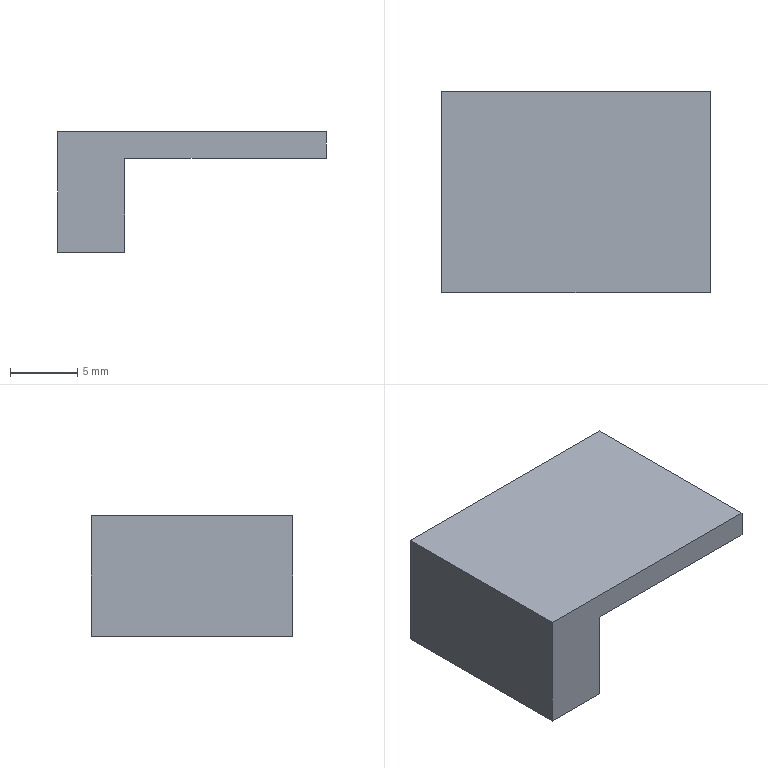Part | SolidWorks | features Extrusion 1, ICE 1 | 1 solid | 8 faces | box 20 x 15 x 9 mm | volume 1125 mm3 | plane 8
STEP:
#1=CARTESIAN_POINT('',(2.5,-7.5,0.));
#2=VERTEX_POINT('',#1);
#3=CARTESIAN_POINT('',(2.5,7.5,0.));
#4=VERTEX_POINT('',#3);
#5=CARTESIAN_POINT('',(2.5,7.5,0.));
#6=DIRECTION('',(0.,1.,0.));
#7=VECTOR('',#6,1000.);
#8=LINE('',#5,#7);
#9=EDGE_CURVE('',#2,#4,#8,.T.);
#10=ORIENTED_EDGE('',*,*,#9,.T.);
#11=CARTESIAN_POINT('',(2.5,7.5,7.));
#12=VERTEX_POINT('',#11);
#13=CARTESIAN_POINT('',(2.5,7.5,7.));
#14=DIRECTION('',(0.,0.,-1.));
#15=VECTOR('',#14,1000.);
#16=LINE('',#13,#15);
#17=EDGE_CURVE('',#12,#4,#16,.T.);
#18=ORIENTED_EDGE('',*,*,#17,.F.);
#19=CARTESIAN_POINT('',(2.5,-7.5,7.));
#20=VERTEX_POINT('',#19);
#21=CARTESIAN_POINT('',(2.5,7.5,7.));
#22=DIRECTION('',(0.,1.,0.));
#23=VECTOR('',#22,1000.);
#24=LINE('',#21,#23);
#25=EDGE_CURVE('',#20,#12,#24,.T.);
#26=ORIENTED_EDGE('',*,*,#25,.F.);
#27=CARTESIAN_POINT('',(2.5,-7.5,7.));
#28=DIRECTION('',(0.,0.,-1.));
#29=VECTOR('',#28,1000.);
#30=LINE('',#27,#29);
#31=EDGE_CURVE('',#20,#2,#30,.T.);
#32=ORIENTED_EDGE('',*,*,#31,.T.);
#33=EDGE_LOOP('',(#10,#18,#26,#32));
#34=FACE_OUTER_BOUND('',#33,.T.);
#35=CARTESIAN_POINT('',(2.5,7.5,7.));
#36=DIRECTION('',(-1.,0.,0.));
#37=DIRECTION('',(0.,-1.,0.));
#38=AXIS2_PLACEMENT_3D('',#35,#36,#37);
#39=PLANE('',#38);
#40=ADVANCED_FACE('',(#34),#39,.F.);
#41=CARTESIAN_POINT('',(-2.5,7.5,0.));
#42=VERTEX_POINT('',#41);
#43=CARTESIAN_POINT('',(-2.5,7.5,0.));
#44=DIRECTION('',(-1.,0.,0.));
#45=VECTOR('',#44,1000.);
#46=LINE('',#43,#45);
#47=EDGE_CURVE('',#4,#42,#46,.T.);
#48=ORIENTED_EDGE('',*,*,#47,.T.);
#49=CARTESIAN_POINT('',(-2.5,7.5,9.));
#50=VERTEX_POINT('',#49);
#51=CARTESIAN_POINT('',(-2.5,7.5,7.));
#52=DIRECTION('',(0.,0.,-1.));
#53=VECTOR('',#52,1000.);
#54=LINE('',#51,#53);
#55=EDGE_CURVE('',#50,#42,#54,.T.);
#56=ORIENTED_EDGE('',*,*,#55,.F.);
#57=CARTESIAN_POINT('',(17.5,7.5,9.));
#58=VERTEX_POINT('',#57);
#59=CARTESIAN_POINT('',(-2.5,7.5,9.));
#60=DIRECTION('',(-1.,0.,0.));
#61=VECTOR('',#60,1000.);
#62=LINE('',#59,#61);
#63=EDGE_CURVE('',#58,#50,#62,.T.);
#64=ORIENTED_EDGE('',*,*,#63,.F.);
#65=CARTESIAN_POINT('',(17.5,7.5,7.));
#66=VERTEX_POINT('',#65);
#67=CARTESIAN_POINT('',(17.5,7.5,9.));
#68=DIRECTION('',(0.,0.,-1.));
#69=VECTOR('',#68,1000.);
#70=LINE('',#67,#69);
#71=EDGE_CURVE('',#58,#66,#70,.T.);
#72=ORIENTED_EDGE('',*,*,#71,.T.);
#73=CARTESIAN_POINT('',(-2.5,7.5,7.));
#74=DIRECTION('',(-1.,0.,0.));
#75=VECTOR('',#74,1000.);
#76=LINE('',#73,#75);
#77=EDGE_CURVE('',#66,#12,#76,.T.);
#78=ORIENTED_EDGE('',*,*,#77,.T.);
#79=ORIENTED_EDGE('',*,*,#17,.T.);
#80=EDGE_LOOP('',(#48,#56,#64,#72,#78,#79));
#81=FACE_OUTER_BOUND('',#80,.T.);
#82=CARTESIAN_POINT('',(-2.5,7.5,7.));
#83=DIRECTION('',(0.,-1.,0.));
#84=DIRECTION('',(0.,0.,-1.));
#85=AXIS2_PLACEMENT_3D('',#82,#83,#84);
#86=PLANE('',#85);
#87=ADVANCED_FACE('',(#81),#86,.F.);
#88=CARTESIAN_POINT('',(-2.5,-7.5,0.));
#89=VERTEX_POINT('',#88);
#90=CARTESIAN_POINT('',(-2.5,7.5,0.));
#91=DIRECTION('',(0.,-1.,0.));
#92=VECTOR('',#91,1000.);
#93=LINE('',#90,#92);
#94=EDGE_CURVE('',#42,#89,#93,.T.);
#95=ORIENTED_EDGE('',*,*,#94,.T.);
#96=CARTESIAN_POINT('',(-2.5,-7.5,9.));
#97=VERTEX_POINT('',#96);
#98=CARTESIAN_POINT('',(-2.5,-7.5,7.));
#99=DIRECTION('',(0.,0.,-1.));
#100=VECTOR('',#99,1000.);
#101=LINE('',#98,#100);
#102=EDGE_CURVE('',#97,#89,#101,.T.);
#103=ORIENTED_EDGE('',*,*,#102,.F.);
#104=CARTESIAN_POINT('',(-2.5,7.5,9.));
#105=DIRECTION('',(0.,-1.,0.));
#106=VECTOR('',#105,1000.);
#107=LINE('',#104,#106);
#108=EDGE_CURVE('',#50,#97,#107,.T.);
#109=ORIENTED_EDGE('',*,*,#108,.F.);
#110=ORIENTED_EDGE('',*,*,#55,.T.);
#111=EDGE_LOOP('',(#95,#103,#109,#110));
#112=FACE_OUTER_BOUND('',#111,.T.);
#113=CARTESIAN_POINT('',(-2.5,7.5,7.));
#114=DIRECTION('',(1.,0.,0.));
#115=DIRECTION('',(0.,1.,0.));
#116=AXIS2_PLACEMENT_3D('',#113,#114,#115);
#117=PLANE('',#116);
#118=ADVANCED_FACE('',(#112),#117,.F.);
#119=CARTESIAN_POINT('',(-2.5,-7.5,0.));
#120=DIRECTION('',(1.,0.,0.));
#121=VECTOR('',#120,1000.);
#122=LINE('',#119,#121);
#123=EDGE_CURVE('',#89,#2,#122,.T.);
#124=ORIENTED_EDGE('',*,*,#123,.T.);
#125=ORIENTED_EDGE('',*,*,#31,.F.);
#126=CARTESIAN_POINT('',(17.5,-7.5,7.));
#127=VERTEX_POINT('',#126);
#128=CARTESIAN_POINT('',(-2.5,-7.5,7.));
#129=DIRECTION('',(1.,0.,0.));
#130=VECTOR('',#129,1000.);
#131=LINE('',#128,#130);
#132=EDGE_CURVE('',#20,#127,#131,.T.);
#133=ORIENTED_EDGE('',*,*,#132,.T.);
#134=CARTESIAN_POINT('',(17.5,-7.5,9.));
#135=VERTEX_POINT('',#134);
#136=CARTESIAN_POINT('',(17.5,-7.5,9.));
#137=DIRECTION('',(0.,0.,-1.));
#138=VECTOR('',#137,1000.);
#139=LINE('',#136,#138);
#140=EDGE_CURVE('',#135,#127,#139,.T.);
#141=ORIENTED_EDGE('',*,*,#140,.F.);
#142=CARTESIAN_POINT('',(-2.5,-7.5,9.));
#143=DIRECTION('',(1.,0.,0.));
#144=VECTOR('',#143,1000.);
#145=LINE('',#142,#144);
#146=EDGE_CURVE('',#97,#135,#145,.T.);
#147=ORIENTED_EDGE('',*,*,#146,.F.);
#148=ORIENTED_EDGE('',*,*,#102,.T.);
#149=EDGE_LOOP('',(#124,#125,#133,#141,#147,#148));
#150=FACE_OUTER_BOUND('',#149,.T.);
#151=CARTESIAN_POINT('',(-2.5,-7.5,7.));
#152=DIRECTION('',(0.,1.,0.));
#153=DIRECTION('',(0.,0.,1.));
#154=AXIS2_PLACEMENT_3D('',#151,#152,#153);
#155=PLANE('',#154);
#156=ADVANCED_FACE('',(#150),#155,.F.);
#157=ORIENTED_EDGE('',*,*,#9,.F.);
#158=ORIENTED_EDGE('',*,*,#123,.F.);
#159=ORIENTED_EDGE('',*,*,#94,.F.);
#160=ORIENTED_EDGE('',*,*,#47,.F.);
#161=EDGE_LOOP('',(#157,#158,#159,#160));
#162=FACE_OUTER_BOUND('',#161,.T.);
#163=CARTESIAN_POINT('',(0.,0.,0.));
#164=DIRECTION('',(0.,0.,1.));
#165=DIRECTION('',(1.,0.,0.));
#166=AXIS2_PLACEMENT_3D('',#163,#164,#165);
#167=PLANE('',#166);
#168=ADVANCED_FACE('',(#162),#167,.F.);
#169=ORIENTED_EDGE('',*,*,#132,.F.);
#170=ORIENTED_EDGE('',*,*,#25,.T.);
#171=ORIENTED_EDGE('',*,*,#77,.F.);
#172=CARTESIAN_POINT('',(17.5,7.5,7.));
#173=DIRECTION('',(0.,1.,0.));
#174=VECTOR('',#173,1000.);
#175=LINE('',#172,#174);
#176=EDGE_CURVE('',#127,#66,#175,.T.);
#177=ORIENTED_EDGE('',*,*,#176,.F.);
#178=EDGE_LOOP('',(#169,#170,#171,#177));
#179=FACE_OUTER_BOUND('',#178,.T.);
#180=CARTESIAN_POINT('',(0.,0.,7.));
#181=DIRECTION('',(0.,0.,1.));
#182=DIRECTION('',(1.,0.,0.));
#183=AXIS2_PLACEMENT_3D('',#180,#181,#182);
#184=PLANE('',#183);
#185=ADVANCED_FACE('',(#179),#184,.F.);
#186=ORIENTED_EDGE('',*,*,#176,.T.);
#187=ORIENTED_EDGE('',*,*,#71,.F.);
#188=CARTESIAN_POINT('',(17.5,7.5,9.));
#189=DIRECTION('',(0.,1.,0.));
#190=VECTOR('',#189,1000.);
#191=LINE('',#188,#190);
#192=EDGE_CURVE('',#135,#58,#191,.T.);
#193=ORIENTED_EDGE('',*,*,#192,.F.);
#194=ORIENTED_EDGE('',*,*,#140,.T.);
#195=EDGE_LOOP('',(#186,#187,#193,#194));
#196=FACE_OUTER_BOUND('',#195,.T.);
#197=CARTESIAN_POINT('',(17.5,7.5,9.));
#198=DIRECTION('',(-1.,0.,0.));
#199=DIRECTION('',(0.,0.,1.));
#200=AXIS2_PLACEMENT_3D('',#197,#198,#199);
#201=PLANE('',#200);
#202=ADVANCED_FACE('',(#196),#201,.F.);
#203=ORIENTED_EDGE('',*,*,#108,.T.);
#204=ORIENTED_EDGE('',*,*,#146,.T.);
#205=ORIENTED_EDGE('',*,*,#192,.T.);
#206=ORIENTED_EDGE('',*,*,#63,.T.);
#207=EDGE_LOOP('',(#203,#204,#205,#206));
#208=FACE_OUTER_BOUND('',#207,.T.);
#209=CARTESIAN_POINT('',(0.,0.,9.));
#210=DIRECTION('',(0.,0.,1.));
#211=DIRECTION('',(1.,0.,0.));
#212=AXIS2_PLACEMENT_3D('',#209,#210,#211);
#213=PLANE('',#212);
#214=ADVANCED_FACE('',(#208),#213,.T.);
#215=CLOSED_SHELL('',(#40,#87,#118,#156,#168,#185,#202,#214));
#216=MANIFOLD_SOLID_BREP('',#215);
#217=CARTESIAN_POINT('',(0.,0.,0.));
#218=DIRECTION('',(0.,0.,1.));
#219=DIRECTION('',(1.,0.,0.));
#220=AXIS2_PLACEMENT_3D('',#217,#218,#219);
#221=(LENGTH_UNIT()NAMED_UNIT(*)SI_UNIT(.MILLI.,.METRE.));
#222=UNCERTAINTY_MEASURE_WITH_UNIT(LENGTH_MEASURE(0.00001),#221,'','');
#223=(NAMED_UNIT(*)PLANE_ANGLE_UNIT()SI_UNIT($,.RADIAN.));
#224=(NAMED_UNIT(*)SI_UNIT($,.STERADIAN.)SOLID_ANGLE_UNIT());
#225=(GEOMETRIC_REPRESENTATION_CONTEXT(3)GLOBAL_UNCERTAINTY_ASSIGNED_CONTEXT((#222))GLOBAL_UNIT_ASSIGNED_CONTEXT((#221,#223,#224))REPRESENTATION_CONTEXT('',''));
#226=ADVANCED_BREP_SHAPE_REPRESENTATION('',(#216,#220),#225);